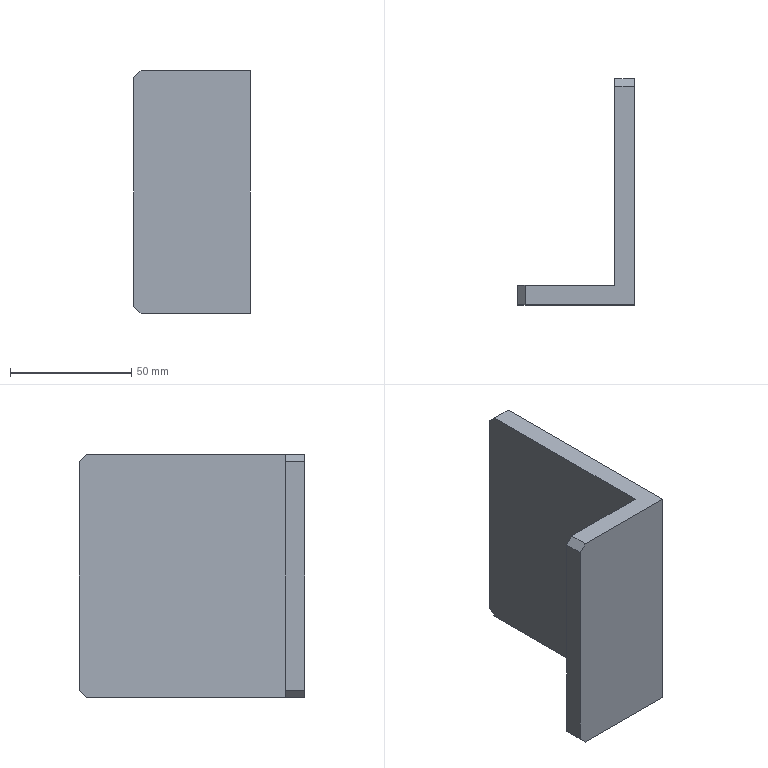Part | SolidWorks | features Chamfer 1, Extrusion 1 | 1 solid | 12 faces | box 48 x 93 x 100 mm | volume 106256 mm3 | plane 12
STEP:
#1=CARTESIAN_POINT('',(-8.,93.,12.621));
#2=VERTEX_POINT('',#1);
#3=CARTESIAN_POINT('',(-8.,93.,-81.379));
#4=VERTEX_POINT('',#3);
#5=CARTESIAN_POINT('',(-8.,93.,15.621));
#6=DIRECTION('',(0.,0.,-1.));
#7=VECTOR('',#6,1000.);
#8=LINE('',#5,#7);
#9=EDGE_CURVE('',#2,#4,#8,.T.);
#10=ORIENTED_EDGE('',*,*,#9,.F.);
#11=CARTESIAN_POINT('',(0.,93.,12.621));
#12=VERTEX_POINT('',#11);
#13=CARTESIAN_POINT('',(-8.,93.,12.621));
#14=DIRECTION('',(1.,0.,0.));
#15=VECTOR('',#14,1000.);
#16=LINE('',#13,#15);
#17=EDGE_CURVE('',#2,#12,#16,.T.);
#18=ORIENTED_EDGE('',*,*,#17,.T.);
#19=CARTESIAN_POINT('',(0.,93.,-81.379));
#20=VERTEX_POINT('',#19);
#21=CARTESIAN_POINT('',(0.,93.,15.621));
#22=DIRECTION('',(0.,0.,-1.));
#23=VECTOR('',#22,1000.);
#24=LINE('',#21,#23);
#25=EDGE_CURVE('',#12,#20,#24,.T.);
#26=ORIENTED_EDGE('',*,*,#25,.T.);
#27=CARTESIAN_POINT('',(-8.,93.,-81.379));
#28=DIRECTION('',(-1.,0.,0.));
#29=VECTOR('',#28,1000.);
#30=LINE('',#27,#29);
#31=EDGE_CURVE('',#20,#4,#30,.T.);
#32=ORIENTED_EDGE('',*,*,#31,.T.);
#33=EDGE_LOOP('',(#10,#18,#26,#32));
#34=FACE_OUTER_BOUND('',#33,.T.);
#35=CARTESIAN_POINT('',(-8.,93.,15.621));
#36=DIRECTION('',(0.,-1.,0.));
#37=DIRECTION('',(0.,0.,-1.));
#38=AXIS2_PLACEMENT_3D('',#35,#36,#37);
#39=PLANE('',#38);
#40=ADVANCED_FACE('',(#34),#39,.F.);
#41=CARTESIAN_POINT('',(-8.,90.,15.621));
#42=VERTEX_POINT('',#41);
#43=CARTESIAN_POINT('',(-8.,8.,15.621));
#44=VERTEX_POINT('',#43);
#45=CARTESIAN_POINT('',(-8.,8.,15.621));
#46=DIRECTION('',(0.,-1.,0.));
#47=VECTOR('',#46,1000.);
#48=LINE('',#45,#47);
#49=EDGE_CURVE('',#42,#44,#48,.T.);
#50=ORIENTED_EDGE('',*,*,#49,.F.);
#51=CARTESIAN_POINT('',(-8.,90.,15.621));
#52=DIRECTION('',(0.,0.7071,-0.7071));
#53=VECTOR('',#52,1000.);
#54=LINE('',#51,#53);
#55=EDGE_CURVE('',#42,#2,#54,.T.);
#56=ORIENTED_EDGE('',*,*,#55,.T.);
#57=ORIENTED_EDGE('',*,*,#9,.T.);
#58=CARTESIAN_POINT('',(-8.,90.,-84.379));
#59=VERTEX_POINT('',#58);
#60=CARTESIAN_POINT('',(-8.,93.,-81.379));
#61=DIRECTION('',(0.,-0.7071,-0.7071));
#62=VECTOR('',#61,1000.);
#63=LINE('',#60,#62);
#64=EDGE_CURVE('',#4,#59,#63,.T.);
#65=ORIENTED_EDGE('',*,*,#64,.T.);
#66=CARTESIAN_POINT('',(-8.,8.,-84.379));
#67=VERTEX_POINT('',#66);
#68=CARTESIAN_POINT('',(-8.,8.,-84.379));
#69=DIRECTION('',(0.,-1.,0.));
#70=VECTOR('',#69,1000.);
#71=LINE('',#68,#70);
#72=EDGE_CURVE('',#59,#67,#71,.T.);
#73=ORIENTED_EDGE('',*,*,#72,.T.);
#74=CARTESIAN_POINT('',(-8.,8.,15.621));
#75=DIRECTION('',(0.,0.,-1.));
#76=VECTOR('',#75,1000.);
#77=LINE('',#74,#76);
#78=EDGE_CURVE('',#44,#67,#77,.T.);
#79=ORIENTED_EDGE('',*,*,#78,.F.);
#80=EDGE_LOOP('',(#50,#56,#57,#65,#73,#79));
#81=FACE_OUTER_BOUND('',#80,.T.);
#82=CARTESIAN_POINT('',(-8.,8.,15.621));
#83=DIRECTION('',(1.,0.,0.));
#84=DIRECTION('',(0.,0.,-1.));
#85=AXIS2_PLACEMENT_3D('',#82,#83,#84);
#86=PLANE('',#85);
#87=ADVANCED_FACE('',(#81),#86,.F.);
#88=CARTESIAN_POINT('',(-45.,8.,-84.379));
#89=VERTEX_POINT('',#88);
#90=CARTESIAN_POINT('',(-48.,8.,-84.379));
#91=DIRECTION('',(-1.,0.,0.));
#92=VECTOR('',#91,1000.);
#93=LINE('',#90,#92);
#94=EDGE_CURVE('',#67,#89,#93,.T.);
#95=ORIENTED_EDGE('',*,*,#94,.T.);
#96=CARTESIAN_POINT('',(-48.,8.,-81.379));
#97=VERTEX_POINT('',#96);
#98=CARTESIAN_POINT('',(-48.,8.,-81.379));
#99=DIRECTION('',(-0.7071,0.,0.7071));
#100=VECTOR('',#99,1000.);
#101=LINE('',#98,#100);
#102=EDGE_CURVE('',#89,#97,#101,.T.);
#103=ORIENTED_EDGE('',*,*,#102,.T.);
#104=CARTESIAN_POINT('',(-48.,8.,12.621));
#105=VERTEX_POINT('',#104);
#106=CARTESIAN_POINT('',(-48.,8.,15.621));
#107=DIRECTION('',(0.,0.,-1.));
#108=VECTOR('',#107,1000.);
#109=LINE('',#106,#108);
#110=EDGE_CURVE('',#105,#97,#109,.T.);
#111=ORIENTED_EDGE('',*,*,#110,.F.);
#112=CARTESIAN_POINT('',(-45.,8.,15.621));
#113=VERTEX_POINT('',#112);
#114=CARTESIAN_POINT('',(-45.,8.,15.621));
#115=DIRECTION('',(0.7071,0.,0.7071));
#116=VECTOR('',#115,1000.);
#117=LINE('',#114,#116);
#118=EDGE_CURVE('',#105,#113,#117,.T.);
#119=ORIENTED_EDGE('',*,*,#118,.T.);
#120=CARTESIAN_POINT('',(-48.,8.,15.621));
#121=DIRECTION('',(-1.,0.,0.));
#122=VECTOR('',#121,1000.);
#123=LINE('',#120,#122);
#124=EDGE_CURVE('',#44,#113,#123,.T.);
#125=ORIENTED_EDGE('',*,*,#124,.F.);
#126=ORIENTED_EDGE('',*,*,#78,.T.);
#127=EDGE_LOOP('',(#95,#103,#111,#119,#125,#126));
#128=FACE_OUTER_BOUND('',#127,.T.);
#129=CARTESIAN_POINT('',(-48.,8.,15.621));
#130=DIRECTION('',(0.,-1.,0.));
#131=DIRECTION('',(1.,0.,0.));
#132=AXIS2_PLACEMENT_3D('',#129,#130,#131);
#133=PLANE('',#132);
#134=ADVANCED_FACE('',(#128),#133,.F.);
#135=ORIENTED_EDGE('',*,*,#110,.T.);
#136=CARTESIAN_POINT('',(-48.,0.,-81.379));
#137=VERTEX_POINT('',#136);
#138=CARTESIAN_POINT('',(-48.,0.,-81.379));
#139=DIRECTION('',(0.,-1.,0.));
#140=VECTOR('',#139,1000.);
#141=LINE('',#138,#140);
#142=EDGE_CURVE('',#97,#137,#141,.T.);
#143=ORIENTED_EDGE('',*,*,#142,.T.);
#144=CARTESIAN_POINT('',(-48.,0.,12.621));
#145=VERTEX_POINT('',#144);
#146=CARTESIAN_POINT('',(-48.,0.,15.621));
#147=DIRECTION('',(0.,0.,-1.));
#148=VECTOR('',#147,1000.);
#149=LINE('',#146,#148);
#150=EDGE_CURVE('',#145,#137,#149,.T.);
#151=ORIENTED_EDGE('',*,*,#150,.F.);
#152=CARTESIAN_POINT('',(-48.,0.,12.621));
#153=DIRECTION('',(0.,1.,0.));
#154=VECTOR('',#153,1000.);
#155=LINE('',#152,#154);
#156=EDGE_CURVE('',#145,#105,#155,.T.);
#157=ORIENTED_EDGE('',*,*,#156,.T.);
#158=EDGE_LOOP('',(#135,#143,#151,#157));
#159=FACE_OUTER_BOUND('',#158,.T.);
#160=CARTESIAN_POINT('',(-48.,0.,15.621));
#161=DIRECTION('',(1.,0.,0.));
#162=DIRECTION('',(0.,0.,-1.));
#163=AXIS2_PLACEMENT_3D('',#160,#161,#162);
#164=PLANE('',#163);
#165=ADVANCED_FACE('',(#159),#164,.F.);
#166=ORIENTED_EDGE('',*,*,#150,.T.);
#167=CARTESIAN_POINT('',(-45.,0.,-84.379));
#168=VERTEX_POINT('',#167);
#169=CARTESIAN_POINT('',(-48.,0.,-81.379));
#170=DIRECTION('',(0.7071,0.,-0.7071));
#171=VECTOR('',#170,1000.);
#172=LINE('',#169,#171);
#173=EDGE_CURVE('',#137,#168,#172,.T.);
#174=ORIENTED_EDGE('',*,*,#173,.T.);
#175=CARTESIAN_POINT('',(0.,0.,-84.379));
#176=VERTEX_POINT('',#175);
#177=CARTESIAN_POINT('',(0.,0.,-84.379));
#178=DIRECTION('',(1.,0.,0.));
#179=VECTOR('',#178,1000.);
#180=LINE('',#177,#179);
#181=EDGE_CURVE('',#168,#176,#180,.T.);
#182=ORIENTED_EDGE('',*,*,#181,.T.);
#183=CARTESIAN_POINT('',(0.,0.,15.621));
#184=VERTEX_POINT('',#183);
#185=CARTESIAN_POINT('',(0.,0.,15.621));
#186=DIRECTION('',(0.,0.,-1.));
#187=VECTOR('',#186,1000.);
#188=LINE('',#185,#187);
#189=EDGE_CURVE('',#184,#176,#188,.T.);
#190=ORIENTED_EDGE('',*,*,#189,.F.);
#191=CARTESIAN_POINT('',(-45.,0.,15.621));
#192=VERTEX_POINT('',#191);
#193=CARTESIAN_POINT('',(0.,0.,15.621));
#194=DIRECTION('',(1.,0.,0.));
#195=VECTOR('',#194,1000.);
#196=LINE('',#193,#195);
#197=EDGE_CURVE('',#192,#184,#196,.T.);
#198=ORIENTED_EDGE('',*,*,#197,.F.);
#199=CARTESIAN_POINT('',(-45.,0.,15.621));
#200=DIRECTION('',(-0.7071,0.,-0.7071));
#201=VECTOR('',#200,1000.);
#202=LINE('',#199,#201);
#203=EDGE_CURVE('',#192,#145,#202,.T.);
#204=ORIENTED_EDGE('',*,*,#203,.T.);
#205=EDGE_LOOP('',(#166,#174,#182,#190,#198,#204));
#206=FACE_OUTER_BOUND('',#205,.T.);
#207=CARTESIAN_POINT('',(0.,0.,15.621));
#208=DIRECTION('',(0.,1.,0.));
#209=DIRECTION('',(-1.,0.,0.));
#210=AXIS2_PLACEMENT_3D('',#207,#208,#209);
#211=PLANE('',#210);
#212=ADVANCED_FACE('',(#206),#211,.F.);
#213=ORIENTED_EDGE('',*,*,#25,.F.);
#214=CARTESIAN_POINT('',(0.,90.,15.621));
#215=VERTEX_POINT('',#214);
#216=CARTESIAN_POINT('',(0.,90.,15.621));
#217=DIRECTION('',(0.,-0.7071,0.7071));
#218=VECTOR('',#217,1000.);
#219=LINE('',#216,#218);
#220=EDGE_CURVE('',#12,#215,#219,.T.);
#221=ORIENTED_EDGE('',*,*,#220,.T.);
#222=CARTESIAN_POINT('',(0.,93.,15.621));
#223=DIRECTION('',(0.,1.,0.));
#224=VECTOR('',#223,1000.);
#225=LINE('',#222,#224);
#226=EDGE_CURVE('',#184,#215,#225,.T.);
#227=ORIENTED_EDGE('',*,*,#226,.F.);
#228=ORIENTED_EDGE('',*,*,#189,.T.);
#229=CARTESIAN_POINT('',(0.,90.,-84.379));
#230=VERTEX_POINT('',#229);
#231=CARTESIAN_POINT('',(0.,93.,-84.379));
#232=DIRECTION('',(0.,1.,0.));
#233=VECTOR('',#232,1000.);
#234=LINE('',#231,#233);
#235=EDGE_CURVE('',#176,#230,#234,.T.);
#236=ORIENTED_EDGE('',*,*,#235,.T.);
#237=CARTESIAN_POINT('',(0.,93.,-81.379));
#238=DIRECTION('',(0.,0.7071,0.7071));
#239=VECTOR('',#238,1000.);
#240=LINE('',#237,#239);
#241=EDGE_CURVE('',#230,#20,#240,.T.);
#242=ORIENTED_EDGE('',*,*,#241,.T.);
#243=EDGE_LOOP('',(#213,#221,#227,#228,#236,#242));
#244=FACE_OUTER_BOUND('',#243,.T.);
#245=CARTESIAN_POINT('',(0.,93.,15.621));
#246=DIRECTION('',(-1.,0.,0.));
#247=DIRECTION('',(0.,0.,1.));
#248=AXIS2_PLACEMENT_3D('',#245,#246,#247);
#249=PLANE('',#248);
#250=ADVANCED_FACE('',(#244),#249,.F.);
#251=ORIENTED_EDGE('',*,*,#124,.T.);
#252=CARTESIAN_POINT('',(-45.,0.,15.621));
#253=DIRECTION('',(0.,-1.,0.));
#254=VECTOR('',#253,1000.);
#255=LINE('',#252,#254);
#256=EDGE_CURVE('',#113,#192,#255,.T.);
#257=ORIENTED_EDGE('',*,*,#256,.T.);
#258=ORIENTED_EDGE('',*,*,#197,.T.);
#259=ORIENTED_EDGE('',*,*,#226,.T.);
#260=CARTESIAN_POINT('',(0.,90.,15.621));
#261=DIRECTION('',(-1.,0.,0.));
#262=VECTOR('',#261,1000.);
#263=LINE('',#260,#262);
#264=EDGE_CURVE('',#215,#42,#263,.T.);
#265=ORIENTED_EDGE('',*,*,#264,.T.);
#266=ORIENTED_EDGE('',*,*,#49,.T.);
#267=EDGE_LOOP('',(#251,#257,#258,#259,#265,#266));
#268=FACE_OUTER_BOUND('',#267,.T.);
#269=CARTESIAN_POINT('',(0.,0.,15.621));
#270=DIRECTION('',(0.,0.,-1.));
#271=DIRECTION('',(-1.,0.,0.));
#272=AXIS2_PLACEMENT_3D('',#269,#270,#271);
#273=PLANE('',#272);
#274=ADVANCED_FACE('',(#268),#273,.F.);
#275=ORIENTED_EDGE('',*,*,#181,.F.);
#276=CARTESIAN_POINT('',(-45.,8.,-84.379));
#277=DIRECTION('',(0.,1.,0.));
#278=VECTOR('',#277,1000.);
#279=LINE('',#276,#278);
#280=EDGE_CURVE('',#168,#89,#279,.T.);
#281=ORIENTED_EDGE('',*,*,#280,.T.);
#282=ORIENTED_EDGE('',*,*,#94,.F.);
#283=ORIENTED_EDGE('',*,*,#72,.F.);
#284=CARTESIAN_POINT('',(0.,90.,-84.379));
#285=DIRECTION('',(1.,0.,0.));
#286=VECTOR('',#285,1000.);
#287=LINE('',#284,#286);
#288=EDGE_CURVE('',#59,#230,#287,.T.);
#289=ORIENTED_EDGE('',*,*,#288,.T.);
#290=ORIENTED_EDGE('',*,*,#235,.F.);
#291=EDGE_LOOP('',(#275,#281,#282,#283,#289,#290));
#292=FACE_OUTER_BOUND('',#291,.T.);
#293=CARTESIAN_POINT('',(0.,0.,-84.379));
#294=DIRECTION('',(0.,0.,-1.));
#295=DIRECTION('',(-1.,0.,0.));
#296=AXIS2_PLACEMENT_3D('',#293,#294,#295);
#297=PLANE('',#296);
#298=ADVANCED_FACE('',(#292),#297,.T.);
#299=ORIENTED_EDGE('',*,*,#102,.F.);
#300=ORIENTED_EDGE('',*,*,#280,.F.);
#301=ORIENTED_EDGE('',*,*,#173,.F.);
#302=ORIENTED_EDGE('',*,*,#142,.F.);
#303=EDGE_LOOP('',(#299,#300,#301,#302));
#304=FACE_OUTER_BOUND('',#303,.T.);
#305=CARTESIAN_POINT('',(-48.,0.,-81.379));
#306=DIRECTION('',(-0.7071,0.,-0.7071));
#307=DIRECTION('',(0.,1.,0.));
#308=AXIS2_PLACEMENT_3D('',#305,#306,#307);
#309=PLANE('',#308);
#310=ADVANCED_FACE('',(#304),#309,.T.);
#311=ORIENTED_EDGE('',*,*,#118,.F.);
#312=ORIENTED_EDGE('',*,*,#156,.F.);
#313=ORIENTED_EDGE('',*,*,#203,.F.);
#314=ORIENTED_EDGE('',*,*,#256,.F.);
#315=EDGE_LOOP('',(#311,#312,#313,#314));
#316=FACE_OUTER_BOUND('',#315,.T.);
#317=CARTESIAN_POINT('',(-45.,0.,15.621));
#318=DIRECTION('',(0.7071,0.,-0.7071));
#319=DIRECTION('',(0.,-1.,0.));
#320=AXIS2_PLACEMENT_3D('',#317,#318,#319);
#321=PLANE('',#320);
#322=ADVANCED_FACE('',(#316),#321,.F.);
#323=ORIENTED_EDGE('',*,*,#220,.F.);
#324=ORIENTED_EDGE('',*,*,#17,.F.);
#325=ORIENTED_EDGE('',*,*,#55,.F.);
#326=ORIENTED_EDGE('',*,*,#264,.F.);
#327=EDGE_LOOP('',(#323,#324,#325,#326));
#328=FACE_OUTER_BOUND('',#327,.T.);
#329=CARTESIAN_POINT('',(0.,90.,15.621));
#330=DIRECTION('',(0.,-0.7071,-0.7071));
#331=DIRECTION('',(-1.,0.,0.));
#332=AXIS2_PLACEMENT_3D('',#329,#330,#331);
#333=PLANE('',#332);
#334=ADVANCED_FACE('',(#328),#333,.F.);
#335=ORIENTED_EDGE('',*,*,#241,.F.);
#336=ORIENTED_EDGE('',*,*,#288,.F.);
#337=ORIENTED_EDGE('',*,*,#64,.F.);
#338=ORIENTED_EDGE('',*,*,#31,.F.);
#339=EDGE_LOOP('',(#335,#336,#337,#338));
#340=FACE_OUTER_BOUND('',#339,.T.);
#341=CARTESIAN_POINT('',(-8.,93.,-81.379));
#342=DIRECTION('',(0.,0.7071,-0.7071));
#343=DIRECTION('',(1.,0.,0.));
#344=AXIS2_PLACEMENT_3D('',#341,#342,#343);
#345=PLANE('',#344);
#346=ADVANCED_FACE('',(#340),#345,.T.);
#347=CLOSED_SHELL('',(#40,#87,#134,#165,#212,#250,#274,#298,#310,#322,#334,#346));
#348=MANIFOLD_SOLID_BREP('',#347);
#349=CARTESIAN_POINT('',(0.,0.,0.));
#350=DIRECTION('',(0.,0.,1.));
#351=DIRECTION('',(1.,0.,0.));
#352=AXIS2_PLACEMENT_3D('',#349,#350,#351);
#353=(LENGTH_UNIT()NAMED_UNIT(*)SI_UNIT(.MILLI.,.METRE.));
#354=UNCERTAINTY_MEASURE_WITH_UNIT(LENGTH_MEASURE(0.00001),#353,'','');
#355=(NAMED_UNIT(*)PLANE_ANGLE_UNIT()SI_UNIT($,.RADIAN.));
#356=(NAMED_UNIT(*)SI_UNIT($,.STERADIAN.)SOLID_ANGLE_UNIT());
#357=(GEOMETRIC_REPRESENTATION_CONTEXT(3)GLOBAL_UNCERTAINTY_ASSIGNED_CONTEXT((#354))GLOBAL_UNIT_ASSIGNED_CONTEXT((#353,#355,#356))REPRESENTATION_CONTEXT('',''));
#358=ADVANCED_BREP_SHAPE_REPRESENTATION('',(#348,#352),#357);